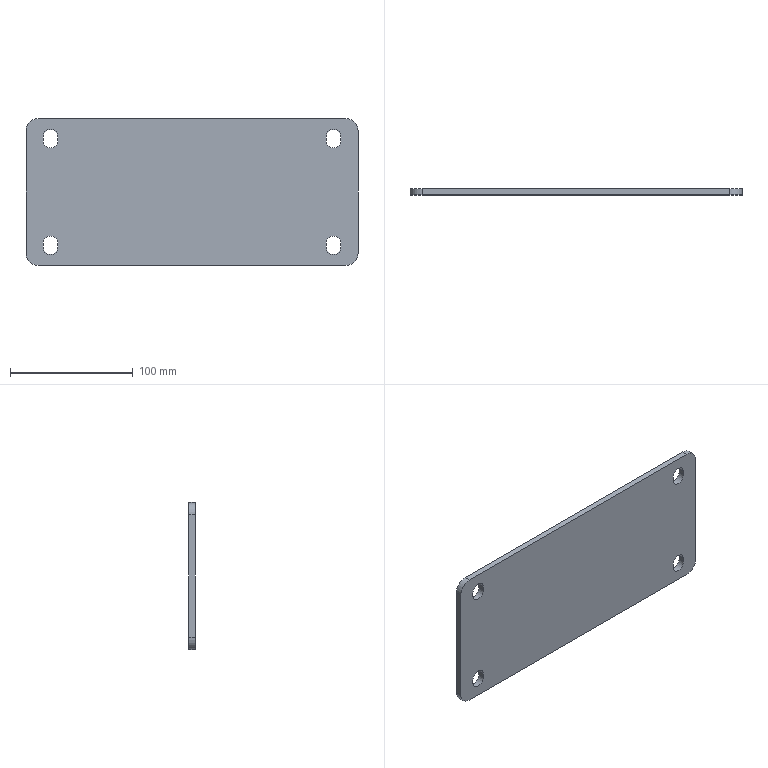Part | STEP file | HL4GD-1.30.102 upper-deck ladder mounting plate--20251212 | 1 solid | 26 faces | box 271 x 5 x 120 mm | volume 159189 mm3 | plane 14 | cylinder 12 | commonest cylinder face diameters 12 x8 20 x4